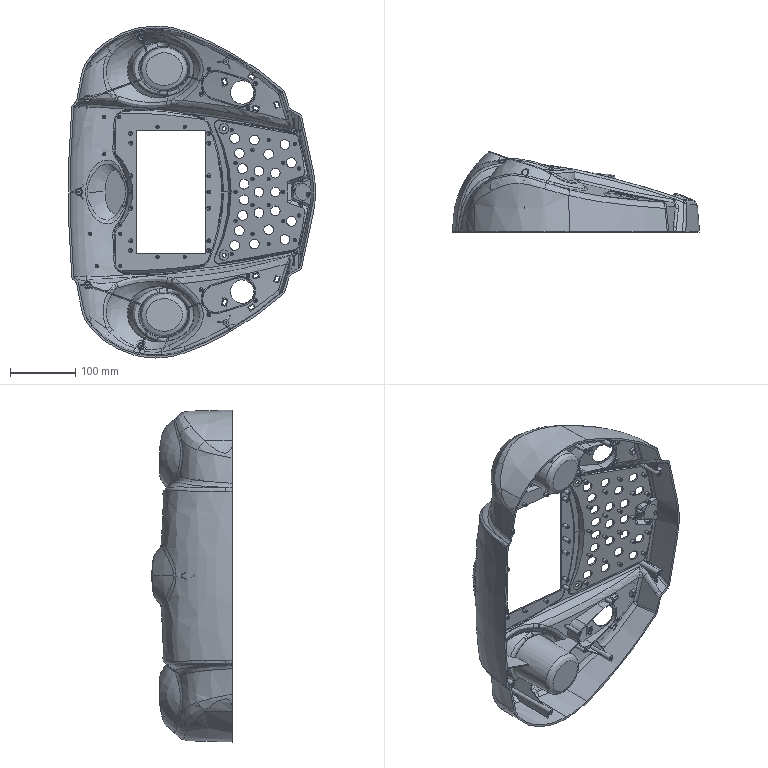Part | STEP file | 6151206W | 1 solid | 1177 faces | box 380 x 123.405 x 510 mm | volume 795942 mm3 | spline 636 | plane 292 | cylinder 160 | cone 70 | torus 17 | sphere 2 | commonest cylinder face diameters 5 x32 6 x27 15 x22 2 x14 8 x10 12 x10